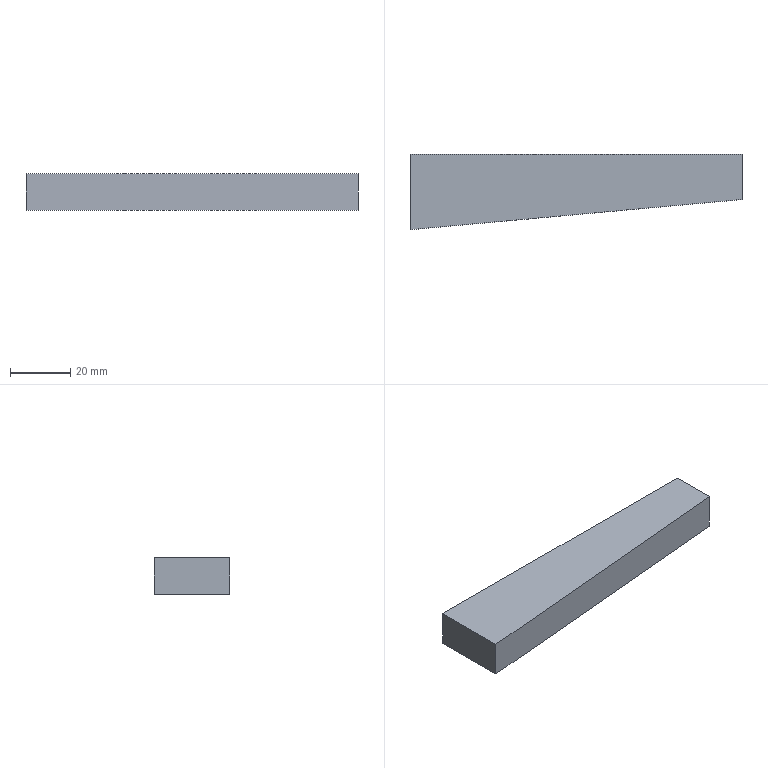Part | STEP file | Positioning_id1802_x_t | 1 solid | 6 faces | box 110 x 25 x 12 mm | volume 26400 mm3 | plane 6
STEP:
#1=CARTESIAN_POINT('',(0.,0.,0.));
#2=DIRECTION('',(0.,0.,1.));
#3=DIRECTION('',(1.,0.,0.));
#4=AXIS2_PLACEMENT_3D('',#1,#2,#3);
#5=CARTESIAN_POINT('',(-793.002,599.,116.002));
#6=VERTEX_POINT('',#5);
#7=CARTESIAN_POINT('',(-683.002,609.,116.002));
#8=VERTEX_POINT('',#7);
#9=CARTESIAN_POINT('',(-793.002,599.,116.002));
#10=DIRECTION('',(0.9959,0.09054,0.));
#11=VECTOR('',#10,1.);
#12=LINE('',#9,#11);
#13=CARTESIAN_POINT('',(-683.002,609.,116.002));
#14=DIRECTION('',(0.09054,-0.9959,0.));
#15=DIRECTION('',(0.9959,0.09054,0.));
#16=AXIS2_PLACEMENT_3D('',#13,#14,#15);
#17=PLANE('',#16);
#18=CARTESIAN_POINT('',(-110.454,0.));
#19=DIRECTION('',(1.,0.));
#20=VECTOR('',#19,1.);
#21=LINE('',#18,#20);
#22=(GEOMETRIC_REPRESENTATION_CONTEXT(2)PARAMETRIC_REPRESENTATION_CONTEXT()REPRESENTATION_CONTEXT('',''));
#23=DEFINITIONAL_REPRESENTATION('',(#21),#22);
#24=PCURVE('',#17,#23);
#25=CARTESIAN_POINT('',(-731.502,594.,116.002));
#26=DIRECTION('',(0.,0.,-1.));
#27=DIRECTION('',(1.,0.,0.));
#28=AXIS2_PLACEMENT_3D('',#25,#26,#27);
#29=PLANE('',#28);
#30=CARTESIAN_POINT('',(-61.5,-5.));
#31=DIRECTION('',(0.9959,-0.09054));
#32=VECTOR('',#31,1.);
#33=LINE('',#30,#32);
#34=(GEOMETRIC_REPRESENTATION_CONTEXT(2)PARAMETRIC_REPRESENTATION_CONTEXT()REPRESENTATION_CONTEXT('',''));
#35=DEFINITIONAL_REPRESENTATION('',(#33),#34);
#36=PCURVE('',#29,#35);
#37=SURFACE_CURVE('',#12,(#24,#36),.PCURVE_S1.);
#38=EDGE_CURVE('',#6,#8,#37,.T.);
#39=ORIENTED_EDGE('',*,*,#38,.T.);
#40=CARTESIAN_POINT('',(-683.002,609.,128.002));
#41=VERTEX_POINT('',#40);
#42=CARTESIAN_POINT('',(-683.002,609.,116.002));
#43=DIRECTION('',(0.,0.,1.));
#44=VECTOR('',#43,1.);
#45=LINE('',#42,#44);
#46=CARTESIAN_POINT('',(0.,0.));
#47=DIRECTION('',(0.,1.));
#48=VECTOR('',#47,1.);
#49=LINE('',#46,#48);
#50=(GEOMETRIC_REPRESENTATION_CONTEXT(2)PARAMETRIC_REPRESENTATION_CONTEXT()REPRESENTATION_CONTEXT('',''));
#51=DEFINITIONAL_REPRESENTATION('',(#49),#50);
#52=PCURVE('',#17,#51);
#53=CARTESIAN_POINT('',(-683.002,594.,116.002));
#54=DIRECTION('',(1.,0.,0.));
#55=DIRECTION('',(0.,0.,1.));
#56=AXIS2_PLACEMENT_3D('',#53,#54,#55);
#57=PLANE('',#56);
#58=CARTESIAN_POINT('',(0.,-15.));
#59=DIRECTION('',(1.,0.));
#60=VECTOR('',#59,1.);
#61=LINE('',#58,#60);
#62=(GEOMETRIC_REPRESENTATION_CONTEXT(2)PARAMETRIC_REPRESENTATION_CONTEXT()REPRESENTATION_CONTEXT('',''));
#63=DEFINITIONAL_REPRESENTATION('',(#61),#62);
#64=PCURVE('',#57,#63);
#65=SURFACE_CURVE('',#45,(#52,#64),.PCURVE_S1.);
#66=EDGE_CURVE('',#8,#41,#65,.T.);
#67=ORIENTED_EDGE('',*,*,#66,.T.);
#68=CARTESIAN_POINT('',(-793.002,599.,128.002));
#69=VERTEX_POINT('',#68);
#70=CARTESIAN_POINT('',(-683.002,609.,128.002));
#71=DIRECTION('',(-0.9959,-0.09054,0.));
#72=VECTOR('',#71,1.);
#73=LINE('',#70,#72);
#74=CARTESIAN_POINT('',(0.,12.));
#75=DIRECTION('',(-1.,0.));
#76=VECTOR('',#75,1.);
#77=LINE('',#74,#76);
#78=(GEOMETRIC_REPRESENTATION_CONTEXT(2)PARAMETRIC_REPRESENTATION_CONTEXT()REPRESENTATION_CONTEXT('',''));
#79=DEFINITIONAL_REPRESENTATION('',(#77),#78);
#80=PCURVE('',#17,#79);
#81=CARTESIAN_POINT('',(-731.502,594.,128.002));
#82=DIRECTION('',(0.,0.,-1.));
#83=DIRECTION('',(1.,0.,0.));
#84=AXIS2_PLACEMENT_3D('',#81,#82,#83);
#85=PLANE('',#84);
#86=CARTESIAN_POINT('',(48.5,-15.));
#87=DIRECTION('',(-0.9959,0.09054));
#88=VECTOR('',#87,1.);
#89=LINE('',#86,#88);
#90=(GEOMETRIC_REPRESENTATION_CONTEXT(2)PARAMETRIC_REPRESENTATION_CONTEXT()REPRESENTATION_CONTEXT('',''));
#91=DEFINITIONAL_REPRESENTATION('',(#89),#90);
#92=PCURVE('',#85,#91);
#93=SURFACE_CURVE('',#73,(#80,#92),.PCURVE_S1.);
#94=EDGE_CURVE('',#41,#69,#93,.T.);
#95=ORIENTED_EDGE('',*,*,#94,.T.);
#96=CARTESIAN_POINT('',(-793.002,599.,116.002));
#97=DIRECTION('',(0.,0.,1.));
#98=VECTOR('',#97,1.);
#99=LINE('',#96,#98);
#100=CARTESIAN_POINT('',(-110.454,0.));
#101=DIRECTION('',(0.,1.));
#102=VECTOR('',#101,1.);
#103=LINE('',#100,#102);
#104=(GEOMETRIC_REPRESENTATION_CONTEXT(2)PARAMETRIC_REPRESENTATION_CONTEXT()REPRESENTATION_CONTEXT('',''));
#105=DEFINITIONAL_REPRESENTATION('',(#103),#104);
#106=PCURVE('',#17,#105);
#107=CARTESIAN_POINT('',(-793.002,594.,116.002));
#108=DIRECTION('',(1.,0.,0.));
#109=DIRECTION('',(0.,0.,1.));
#110=AXIS2_PLACEMENT_3D('',#107,#108,#109);
#111=PLANE('',#110);
#112=CARTESIAN_POINT('',(0.,-5.));
#113=DIRECTION('',(1.,0.));
#114=VECTOR('',#113,1.);
#115=LINE('',#112,#114);
#116=(GEOMETRIC_REPRESENTATION_CONTEXT(2)PARAMETRIC_REPRESENTATION_CONTEXT()REPRESENTATION_CONTEXT('',''));
#117=DEFINITIONAL_REPRESENTATION('',(#115),#116);
#118=PCURVE('',#111,#117);
#119=SURFACE_CURVE('',#99,(#106,#118),.PCURVE_S1.);
#120=EDGE_CURVE('',#6,#69,#119,.T.);
#121=ORIENTED_EDGE('',*,*,#120,.F.);
#122=EDGE_LOOP('',(#39,#67,#95,#121));
#123=FACE_BOUND('',#122,.T.);
#124=ADVANCED_FACE('',(#123),#17,.T.);
#125=CARTESIAN_POINT('',(-793.002,624.,128.002));
#126=VERTEX_POINT('',#125);
#127=CARTESIAN_POINT('',(-683.002,624.,128.002));
#128=VERTEX_POINT('',#127);
#129=CARTESIAN_POINT('',(-793.002,624.,128.002));
#130=DIRECTION('',(1.,0.,0.));
#131=VECTOR('',#130,1.);
#132=LINE('',#129,#131);
#133=CARTESIAN_POINT('',(-731.502,624.,116.002));
#134=DIRECTION('',(0.,1.,0.));
#135=DIRECTION('',(-1.,0.,0.));
#136=AXIS2_PLACEMENT_3D('',#133,#134,#135);
#137=PLANE('',#136);
#138=CARTESIAN_POINT('',(61.5,12.));
#139=DIRECTION('',(-1.,0.));
#140=VECTOR('',#139,1.);
#141=LINE('',#138,#140);
#142=(GEOMETRIC_REPRESENTATION_CONTEXT(2)PARAMETRIC_REPRESENTATION_CONTEXT()REPRESENTATION_CONTEXT('',''));
#143=DEFINITIONAL_REPRESENTATION('',(#141),#142);
#144=PCURVE('',#137,#143);
#145=CARTESIAN_POINT('',(-61.5,-30.));
#146=DIRECTION('',(1.,0.));
#147=VECTOR('',#146,1.);
#148=LINE('',#145,#147);
#149=(GEOMETRIC_REPRESENTATION_CONTEXT(2)PARAMETRIC_REPRESENTATION_CONTEXT()REPRESENTATION_CONTEXT('',''));
#150=DEFINITIONAL_REPRESENTATION('',(#148),#149);
#151=PCURVE('',#85,#150);
#152=SURFACE_CURVE('',#132,(#144,#151),.PCURVE_S1.);
#153=EDGE_CURVE('',#126,#128,#152,.T.);
#154=ORIENTED_EDGE('',*,*,#153,.T.);
#155=CARTESIAN_POINT('',(-683.002,624.,116.002));
#156=VERTEX_POINT('',#155);
#157=CARTESIAN_POINT('',(-683.002,624.,116.002));
#158=DIRECTION('',(0.,0.,1.));
#159=VECTOR('',#158,1.);
#160=LINE('',#157,#159);
#161=CARTESIAN_POINT('',(-48.5,0.));
#162=DIRECTION('',(0.,1.));
#163=VECTOR('',#162,1.);
#164=LINE('',#161,#163);
#165=(GEOMETRIC_REPRESENTATION_CONTEXT(2)PARAMETRIC_REPRESENTATION_CONTEXT()REPRESENTATION_CONTEXT('',''));
#166=DEFINITIONAL_REPRESENTATION('',(#164),#165);
#167=PCURVE('',#137,#166);
#168=CARTESIAN_POINT('',(0.,-30.));
#169=DIRECTION('',(1.,0.));
#170=VECTOR('',#169,1.);
#171=LINE('',#168,#170);
#172=(GEOMETRIC_REPRESENTATION_CONTEXT(2)PARAMETRIC_REPRESENTATION_CONTEXT()REPRESENTATION_CONTEXT('',''));
#173=DEFINITIONAL_REPRESENTATION('',(#171),#172);
#174=PCURVE('',#57,#173);
#175=SURFACE_CURVE('',#160,(#167,#174),.PCURVE_S1.);
#176=EDGE_CURVE('',#156,#128,#175,.T.);
#177=ORIENTED_EDGE('',*,*,#176,.F.);
#178=CARTESIAN_POINT('',(-793.002,624.,116.002));
#179=VERTEX_POINT('',#178);
#180=CARTESIAN_POINT('',(-793.002,624.,116.002));
#181=DIRECTION('',(1.,0.,0.));
#182=VECTOR('',#181,1.);
#183=LINE('',#180,#182);
#184=CARTESIAN_POINT('',(61.5,0.));
#185=DIRECTION('',(-1.,0.));
#186=VECTOR('',#185,1.);
#187=LINE('',#184,#186);
#188=(GEOMETRIC_REPRESENTATION_CONTEXT(2)PARAMETRIC_REPRESENTATION_CONTEXT()REPRESENTATION_CONTEXT('',''));
#189=DEFINITIONAL_REPRESENTATION('',(#187),#188);
#190=PCURVE('',#137,#189);
#191=CARTESIAN_POINT('',(-61.5,-30.));
#192=DIRECTION('',(1.,0.));
#193=VECTOR('',#192,1.);
#194=LINE('',#191,#193);
#195=(GEOMETRIC_REPRESENTATION_CONTEXT(2)PARAMETRIC_REPRESENTATION_CONTEXT()REPRESENTATION_CONTEXT('',''));
#196=DEFINITIONAL_REPRESENTATION('',(#194),#195);
#197=PCURVE('',#29,#196);
#198=SURFACE_CURVE('',#183,(#190,#197),.PCURVE_S1.);
#199=EDGE_CURVE('',#179,#156,#198,.T.);
#200=ORIENTED_EDGE('',*,*,#199,.F.);
#201=CARTESIAN_POINT('',(-793.002,624.,116.002));
#202=DIRECTION('',(0.,0.,1.));
#203=VECTOR('',#202,1.);
#204=LINE('',#201,#203);
#205=CARTESIAN_POINT('',(61.5,0.));
#206=DIRECTION('',(0.,1.));
#207=VECTOR('',#206,1.);
#208=LINE('',#205,#207);
#209=(GEOMETRIC_REPRESENTATION_CONTEXT(2)PARAMETRIC_REPRESENTATION_CONTEXT()REPRESENTATION_CONTEXT('',''));
#210=DEFINITIONAL_REPRESENTATION('',(#208),#209);
#211=PCURVE('',#137,#210);
#212=CARTESIAN_POINT('',(0.,-30.));
#213=DIRECTION('',(1.,0.));
#214=VECTOR('',#213,1.);
#215=LINE('',#212,#214);
#216=(GEOMETRIC_REPRESENTATION_CONTEXT(2)PARAMETRIC_REPRESENTATION_CONTEXT()REPRESENTATION_CONTEXT('',''));
#217=DEFINITIONAL_REPRESENTATION('',(#215),#216);
#218=PCURVE('',#111,#217);
#219=SURFACE_CURVE('',#204,(#211,#218),.PCURVE_S1.);
#220=EDGE_CURVE('',#179,#126,#219,.T.);
#221=ORIENTED_EDGE('',*,*,#220,.T.);
#222=EDGE_LOOP('',(#154,#177,#200,#221));
#223=FACE_BOUND('',#222,.T.);
#224=ADVANCED_FACE('',(#223),#137,.T.);
#225=ORIENTED_EDGE('',*,*,#220,.F.);
#226=CARTESIAN_POINT('',(-793.002,599.,116.002));
#227=DIRECTION('',(0.,1.,0.));
#228=VECTOR('',#227,1.);
#229=LINE('',#226,#228);
#230=CARTESIAN_POINT('',(0.,-5.));
#231=DIRECTION('',(0.,-1.));
#232=VECTOR('',#231,1.);
#233=LINE('',#230,#232);
#234=(GEOMETRIC_REPRESENTATION_CONTEXT(2)PARAMETRIC_REPRESENTATION_CONTEXT()REPRESENTATION_CONTEXT('',''));
#235=DEFINITIONAL_REPRESENTATION('',(#233),#234);
#236=PCURVE('',#111,#235);
#237=CARTESIAN_POINT('',(-61.5,-5.));
#238=DIRECTION('',(0.,-1.));
#239=VECTOR('',#238,1.);
#240=LINE('',#237,#239);
#241=(GEOMETRIC_REPRESENTATION_CONTEXT(2)PARAMETRIC_REPRESENTATION_CONTEXT()REPRESENTATION_CONTEXT('',''));
#242=DEFINITIONAL_REPRESENTATION('',(#240),#241);
#243=PCURVE('',#29,#242);
#244=SURFACE_CURVE('',#229,(#236,#243),.PCURVE_S1.);
#245=EDGE_CURVE('',#6,#179,#244,.T.);
#246=ORIENTED_EDGE('',*,*,#245,.F.);
#247=ORIENTED_EDGE('',*,*,#120,.T.);
#248=CARTESIAN_POINT('',(-793.002,599.,128.002));
#249=DIRECTION('',(0.,1.,0.));
#250=VECTOR('',#249,1.);
#251=LINE('',#248,#250);
#252=CARTESIAN_POINT('',(12.,-5.));
#253=DIRECTION('',(0.,-1.));
#254=VECTOR('',#253,1.);
#255=LINE('',#252,#254);
#256=(GEOMETRIC_REPRESENTATION_CONTEXT(2)PARAMETRIC_REPRESENTATION_CONTEXT()REPRESENTATION_CONTEXT('',''));
#257=DEFINITIONAL_REPRESENTATION('',(#255),#256);
#258=PCURVE('',#111,#257);
#259=CARTESIAN_POINT('',(-61.5,-5.));
#260=DIRECTION('',(0.,-1.));
#261=VECTOR('',#260,1.);
#262=LINE('',#259,#261);
#263=(GEOMETRIC_REPRESENTATION_CONTEXT(2)PARAMETRIC_REPRESENTATION_CONTEXT()REPRESENTATION_CONTEXT('',''));
#264=DEFINITIONAL_REPRESENTATION('',(#262),#263);
#265=PCURVE('',#85,#264);
#266=SURFACE_CURVE('',#251,(#258,#265),.PCURVE_S1.);
#267=EDGE_CURVE('',#69,#126,#266,.T.);
#268=ORIENTED_EDGE('',*,*,#267,.T.);
#269=EDGE_LOOP('',(#225,#246,#247,#268));
#270=FACE_BOUND('',#269,.T.);
#271=ADVANCED_FACE('',(#270),#111,.F.);
#272=ORIENTED_EDGE('',*,*,#245,.T.);
#273=ORIENTED_EDGE('',*,*,#199,.T.);
#274=CARTESIAN_POINT('',(-683.002,609.,116.002));
#275=DIRECTION('',(0.,1.,0.));
#276=VECTOR('',#275,1.);
#277=LINE('',#274,#276);
#278=CARTESIAN_POINT('',(48.5,-15.));
#279=DIRECTION('',(0.,-1.));
#280=VECTOR('',#279,1.);
#281=LINE('',#278,#280);
#282=(GEOMETRIC_REPRESENTATION_CONTEXT(2)PARAMETRIC_REPRESENTATION_CONTEXT()REPRESENTATION_CONTEXT('',''));
#283=DEFINITIONAL_REPRESENTATION('',(#281),#282);
#284=PCURVE('',#29,#283);
#285=CARTESIAN_POINT('',(0.,-15.));
#286=DIRECTION('',(0.,-1.));
#287=VECTOR('',#286,1.);
#288=LINE('',#285,#287);
#289=(GEOMETRIC_REPRESENTATION_CONTEXT(2)PARAMETRIC_REPRESENTATION_CONTEXT()REPRESENTATION_CONTEXT('',''));
#290=DEFINITIONAL_REPRESENTATION('',(#288),#289);
#291=PCURVE('',#57,#290);
#292=SURFACE_CURVE('',#277,(#284,#291),.PCURVE_S1.);
#293=EDGE_CURVE('',#8,#156,#292,.T.);
#294=ORIENTED_EDGE('',*,*,#293,.F.);
#295=ORIENTED_EDGE('',*,*,#38,.F.);
#296=EDGE_LOOP('',(#272,#273,#294,#295));
#297=FACE_BOUND('',#296,.T.);
#298=ADVANCED_FACE('',(#297),#29,.T.);
#299=ORIENTED_EDGE('',*,*,#293,.T.);
#300=ORIENTED_EDGE('',*,*,#176,.T.);
#301=CARTESIAN_POINT('',(-683.002,609.,128.002));
#302=DIRECTION('',(0.,1.,0.));
#303=VECTOR('',#302,1.);
#304=LINE('',#301,#303);
#305=CARTESIAN_POINT('',(12.,-15.));
#306=DIRECTION('',(0.,-1.));
#307=VECTOR('',#306,1.);
#308=LINE('',#305,#307);
#309=(GEOMETRIC_REPRESENTATION_CONTEXT(2)PARAMETRIC_REPRESENTATION_CONTEXT()REPRESENTATION_CONTEXT('',''));
#310=DEFINITIONAL_REPRESENTATION('',(#308),#309);
#311=PCURVE('',#57,#310);
#312=CARTESIAN_POINT('',(48.5,-15.));
#313=DIRECTION('',(0.,-1.));
#314=VECTOR('',#313,1.);
#315=LINE('',#312,#314);
#316=(GEOMETRIC_REPRESENTATION_CONTEXT(2)PARAMETRIC_REPRESENTATION_CONTEXT()REPRESENTATION_CONTEXT('',''));
#317=DEFINITIONAL_REPRESENTATION('',(#315),#316);
#318=PCURVE('',#85,#317);
#319=SURFACE_CURVE('',#304,(#311,#318),.PCURVE_S1.);
#320=EDGE_CURVE('',#41,#128,#319,.T.);
#321=ORIENTED_EDGE('',*,*,#320,.F.);
#322=ORIENTED_EDGE('',*,*,#66,.F.);
#323=EDGE_LOOP('',(#299,#300,#321,#322));
#324=FACE_BOUND('',#323,.T.);
#325=ADVANCED_FACE('',(#324),#57,.T.);
#326=ORIENTED_EDGE('',*,*,#320,.T.);
#327=ORIENTED_EDGE('',*,*,#153,.F.);
#328=ORIENTED_EDGE('',*,*,#267,.F.);
#329=ORIENTED_EDGE('',*,*,#94,.F.);
#330=EDGE_LOOP('',(#326,#327,#328,#329));
#331=FACE_BOUND('',#330,.T.);
#332=ADVANCED_FACE('',(#331),#85,.F.);
#333=CLOSED_SHELL('',(#124,#224,#271,#298,#325,#332));
#334=MANIFOLD_SOLID_BREP('',#333);
#335=(LENGTH_UNIT()NAMED_UNIT(*)SI_UNIT(.MILLI.,.METRE.));
#336=UNCERTAINTY_MEASURE_WITH_UNIT(LENGTH_MEASURE(0.0000001),#335,'','');
#337=(NAMED_UNIT(*)PLANE_ANGLE_UNIT()SI_UNIT($,.RADIAN.));
#338=(NAMED_UNIT(*)SI_UNIT($,.STERADIAN.)SOLID_ANGLE_UNIT());
#339=(GEOMETRIC_REPRESENTATION_CONTEXT(3)GLOBAL_UNCERTAINTY_ASSIGNED_CONTEXT((#336))GLOBAL_UNIT_ASSIGNED_CONTEXT((#335,#337,#338))REPRESENTATION_CONTEXT('',''));
#340=ADVANCED_BREP_SHAPE_REPRESENTATION('',(#4,#334),#339);